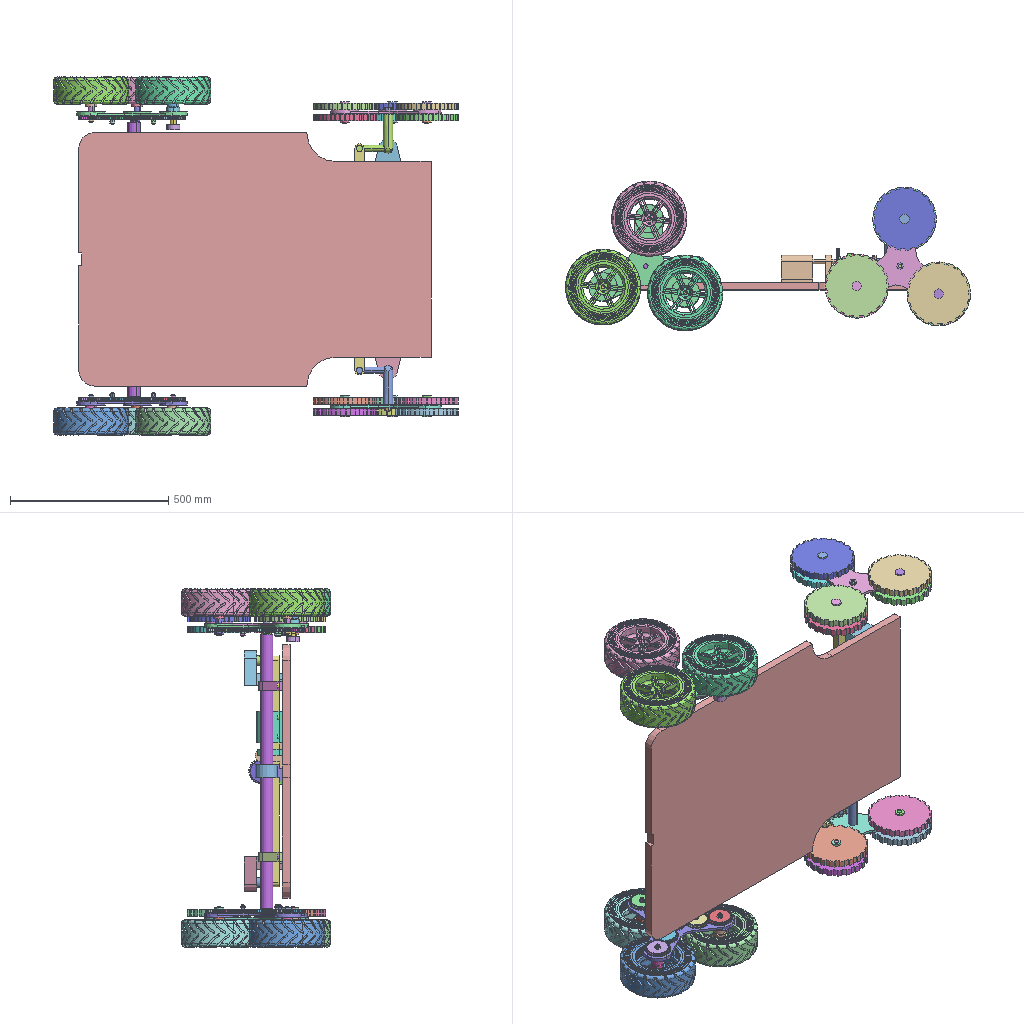Assembly | SolidWorks | 122 different items | 126 placed | box 1278 x 471 x 1130 mm
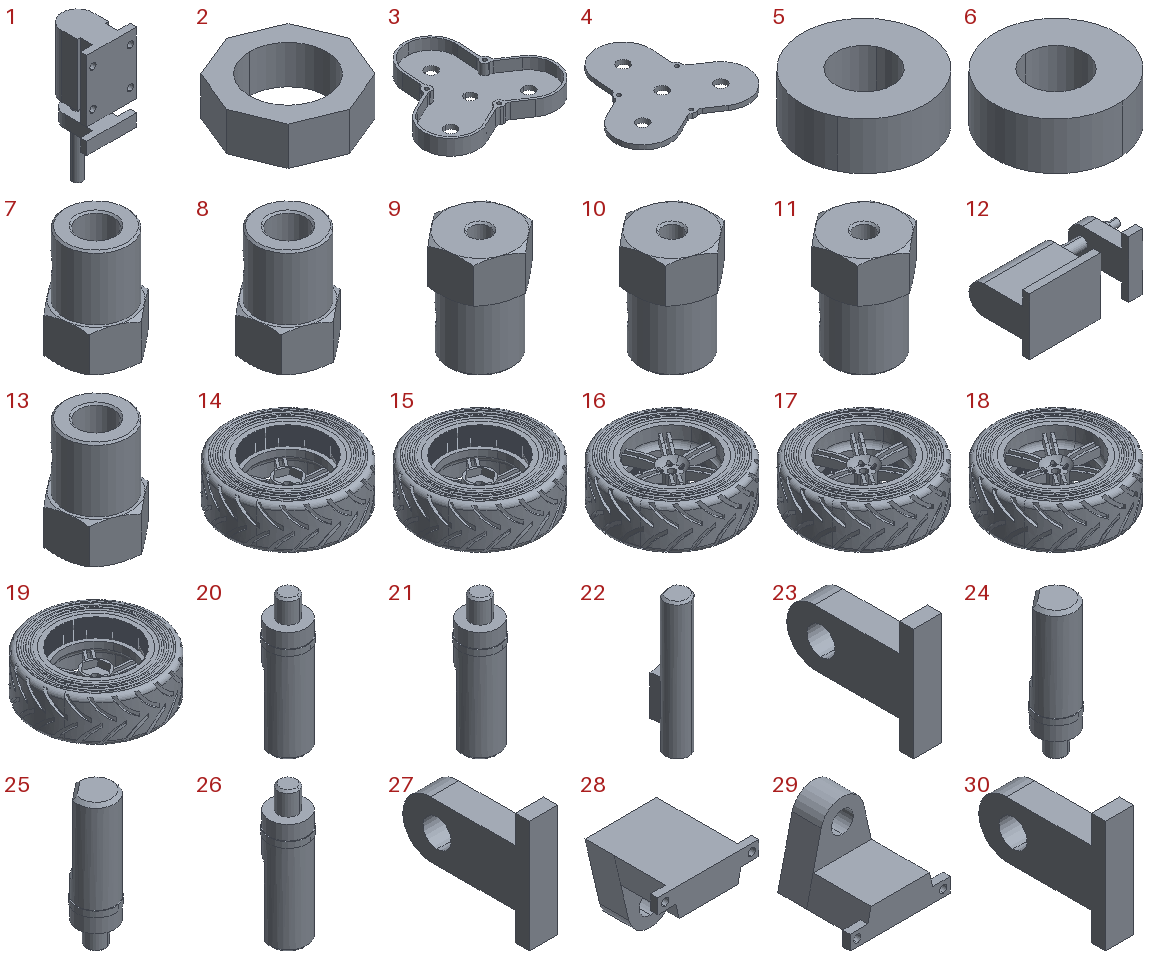Parts list (item | quantity | size | volume | features):
1 | x1 | 80 x 80 x 220 mm | 466808 mm3 | features BaseBody 1
2 | x1 | 16 x 16 x 5 mm | 512.398 mm3 | features BaseBody 1
3 | x1 | 450.446 x 425.125 x 54.4 mm | 2250269 mm3 | features BaseBody 1
4 | x1 | 450.446 x 425.125 x 16 mm | 1740357 mm3 | features BaseBody 1
5 | x1 | 41.6 x 41.6 x 16 mm | 17114 mm3 | features BaseBody 1
6 | x1 | 41.6 x 41.6 x 16 mm | 17114 mm3 | features BaseBody 1
7 | x1 | 41.191 x 43.879 x 57.6 mm | 49620 mm3 | features BaseBody 1
8 | x1 | 41.191 x 43.879 x 57.6 mm | 49620 mm3 | features BaseBody 1
9 | x1 | 41.191 x 43.879 x 57.6 mm | 49620 mm3 | features BaseBody 1
10 | x1 | 41.191 x 43.879 x 57.6 mm | 49620 mm3 | features BaseBody 1
11 | x1 | 41.191 x 43.879 x 57.6 mm | 49620 mm3 | features BaseBody 1
12 | x1 | 188 x 85 x 80 mm | 446040 mm3 | features BaseBody 1
13 | x1 | 41.191 x 43.879 x 57.6 mm | 49620 mm3 | features BaseBody 1
14 | x1 | 236.8 x 236.8 x 86.4 mm | 2369634 mm3 | features BaseBody 1
15 | x1 | 236.8 x 236.8 x 86.4 mm | 2369634 mm3 | features BaseBody 1
16 | x1 | 236.8 x 236.8 x 86.4 mm | 2369635 mm3 | features BaseBody 1
17 | x1 | 236.8 x 236.8 x 86.4 mm | 2369635 mm3 | features BaseBody 1
18 | x1 | 236.8 x 236.8 x 86.4 mm | 2369635 mm3 | features BaseBody 1
19 | x1 | 236.8 x 236.8 x 86.4 mm | 2369634 mm3 | features BaseBody 1
20 | x1 | 20 x 20 x 69.2 mm | 17144 mm3 | features BaseBody 1
21 | x1 | 20 x 20 x 69.2 mm | 17144 mm3 | features BaseBody 1
22 | x1 | 19.2 x 24.894 x 108.8 mm | 33278 mm3 | features BaseBody 1
23 | x1 | 20 x 90 x 80 mm | 70283 mm3 | features BaseBody 1
24 | x1 | 20 x 20 x 69.2 mm | 17144 mm3 | features BaseBody 1
25 | x1 | 20 x 20 x 69.2 mm | 17144 mm3 | features BaseBody 1
26 | x1 | 20 x 20 x 69.2 mm | 17144 mm3 | features BaseBody 1
27 | x1 | 20 x 90 x 80 mm | 70283 mm3 | features BaseBody 1
28 | x1 | 138.517 x 120 x 109.993 mm | 571156 mm3 | features BaseBody 1
29 | x1 | 138.517 x 120 x 109.993 mm | 571156 mm3 | features BaseBody 1
30 | x1 | 20 x 90 x 80 mm | 70283 mm3 | features BaseBody 1
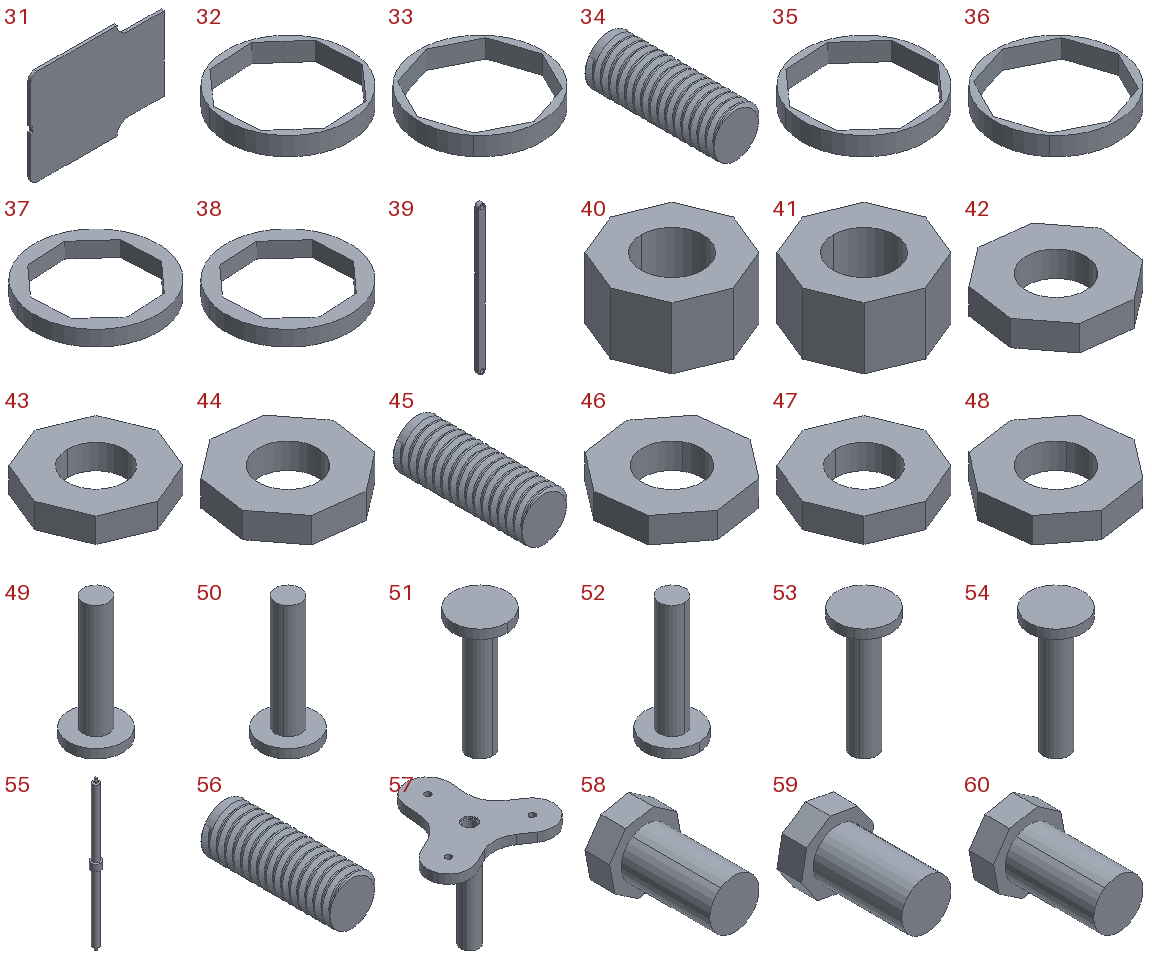31 | x1 | 1112 x 25 x 800 mm | 20489758 mm3 | features BaseBody 1
32 | x1 | 20 x 20 x 3 mm | 176.681 mm3 | features BaseBody 1
33 | x1 | 20 x 20 x 3 mm | 176.681 mm3 | features BaseBody 1
34 | x1 | 6 x 16.008 x 6 mm | 378.104 mm3 | features BaseBody 1
35 | x1 | 20 x 20 x 3 mm | 176.681 mm3 | features BaseBody 1
36 | x1 | 20 x 20 x 3 mm | 176.681 mm3 | features BaseBody 1
37 | x1 | 24 x 24 x 3 mm | 508.64 mm3 | features BaseBody 1
38 | x1 | 24 x 24 x 3 mm | 508.64 mm3 | features BaseBody 1
39 | x1 | 30 x 20 x 730 mm | 420440 mm3 | features BaseBody 1
40 | x1 | 20 x 20 x 10 mm | 2043 mm3 | features BaseBody 1
41 | x1 | 20 x 20 x 10 mm | 2043 mm3 | features BaseBody 1
42 | x1 | 28.978 x 28.978 x 6 mm | 2895 mm3 | features BaseBody 1
43 | x1 | 30 x 30 x 6 mm | 2895 mm3 | features BaseBody 1
44 | x1 | 28.978 x 28.978 x 6 mm | 2895 mm3 | features BaseBody 1
45 | x1 | 6 x 16.008 x 6 mm | 378.104 mm3 | features BaseBody 1
46 | x1 | 28.978 x 28.978 x 6 mm | 2895 mm3 | features BaseBody 1
47 | x1 | 30 x 30 x 6 mm | 2895 mm3 | features BaseBody 1
48 | x1 | 28.978 x 28.978 x 6 mm | 2895 mm3 | features BaseBody 1
49 | x1 | 30 x 30 x 68 mm | 13232 mm3 | features BaseBody 1
50 | x1 | 30 x 30 x 68 mm | 13232 mm3 | features BaseBody 1
51 | x1 | 30 x 30 x 68 mm | 13232 mm3 | features BaseBody 1
52 | x1 | 30 x 30 x 68 mm | 13232 mm3 | features BaseBody 1
53 | x1 | 30 x 30 x 68 mm | 13232 mm3 | features BaseBody 1
54 | x1 | 30 x 30 x 68 mm | 13232 mm3 | features BaseBody 1
55 | x1 | 60 x 60 x 912 mm | 1156729 mm3 | features BaseBody 1
56 | x1 | 6 x 16.008 x 6 mm | 378.104 mm3 | features BaseBody 1
57 | x1 | 199.568 x 186.874 x 175 mm | 351231 mm3 | features BaseBody 1
58 | x1 | 14.681 x 23 x 14.681 mm | 2209 mm3 | features BaseBody 1
59 | x1 | 14.681 x 23 x 14.681 mm | 2209 mm3 | features BaseBody 1
60 | x1 | 14.681 x 23 x 14.681 mm | 2209 mm3 | features BaseBody 1
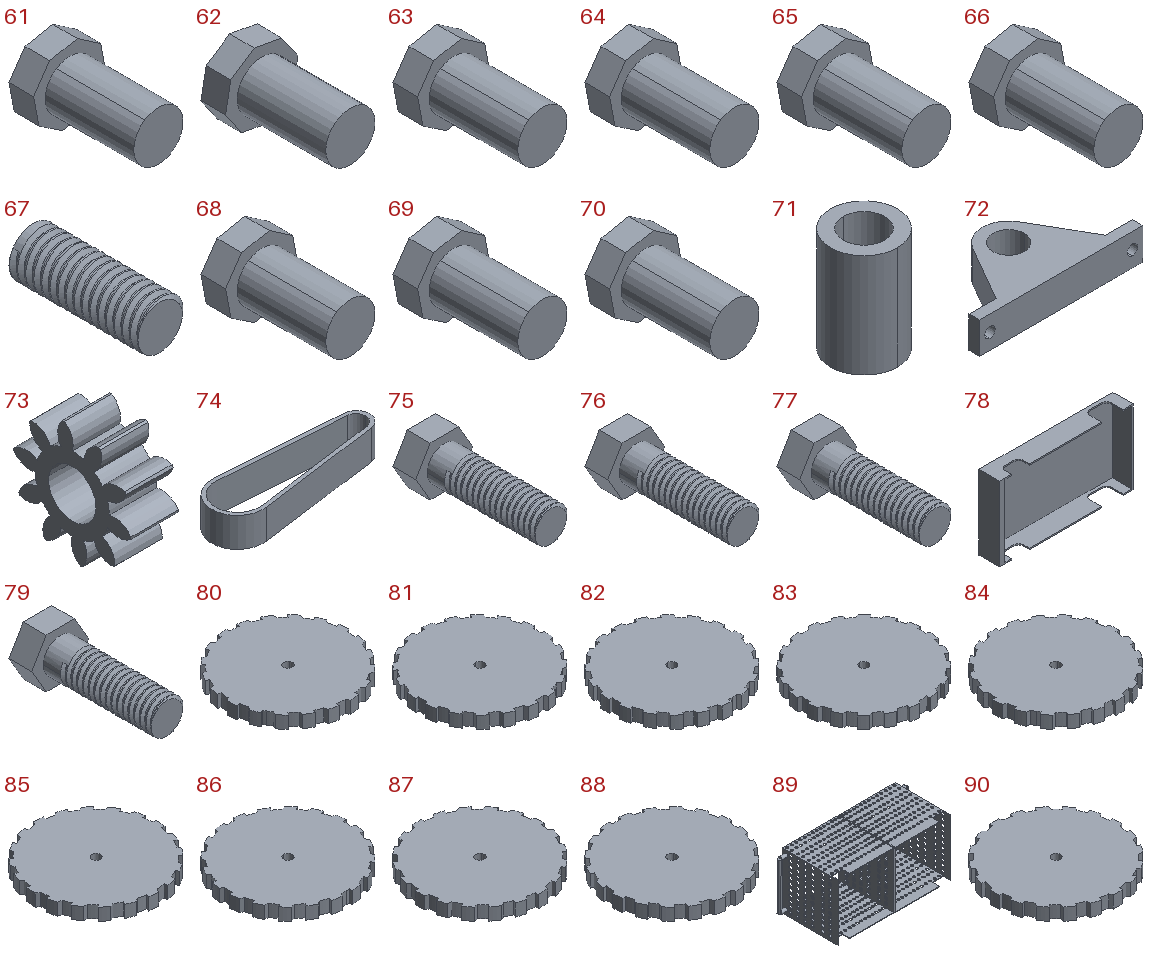61 | x1 | 14.681 x 23 x 14.681 mm | 2209 mm3 | features BaseBody 1
62 | x1 | 14.681 x 23 x 14.681 mm | 2209 mm3 | features BaseBody 1
63 | x1 | 14.681 x 23 x 14.681 mm | 2209 mm3 | features BaseBody 1
64 | x1 | 14.681 x 23 x 14.681 mm | 2209 mm3 | features BaseBody 1
65 | x1 | 14.681 x 23 x 14.681 mm | 2209 mm3 | features BaseBody 1
66 | x1 | 14.681 x 23 x 14.681 mm | 2209 mm3 | features BaseBody 1
67 | x1 | 6 x 16.008 x 6 mm | 378.104 mm3 | features BaseBody 1
68 | x1 | 14.681 x 23 x 14.681 mm | 2209 mm3 | features BaseBody 1
69 | x1 | 14.681 x 23 x 14.681 mm | 2209 mm3 | features BaseBody 1
70 | x1 | 14.681 x 23 x 14.681 mm | 2209 mm3 | features BaseBody 1
71 | x1 | 26 x 26 x 40 mm | 13195 mm3 | features BaseBody 1
72 | x1 | 155.5 x 75 x 30 mm | 151396 mm3 | features BaseBody 1
73 | x1 | - | - | features RefSurface 1
74 | x1 | 219.551 x 70 x 40 mm | 97158 mm3 | features BaseBody 1
75 | x1 | 10 x 23 x 8.66 mm | 722.509 mm3 | features BaseBody 1
76 | x1 | 10 x 23 x 8.66 mm | 722.509 mm3 | features BaseBody 1
77 | x1 | 10 x 23 x 8.66 mm | 722.509 mm3 | features BaseBody 1
78 | x1 | 1112 x 170.835 x 618 mm | 11764605 mm3 | features BaseBody 1
79 | x1 | 10 x 23 x 8.66 mm | 722.509 mm3 | features BaseBody 1
80 | x1 | 199.988 x 199.988 x 20 mm | 595746 mm3 | features BaseBody 1
81 | x1 | 199.75 x 199.75 x 20 mm | 595746 mm3 | features BaseBody 1
82 | x1 | 199.947 x 199.947 x 20 mm | 595746 mm3 | features BaseBody 1
83 | x1 | 199.408 x 199.408 x 20 mm | 595746 mm3 | features BaseBody 1
84 | x1 | 200 x 200 x 20 mm | 595746 mm3 | features BaseBody 1
85 | x1 | 200 x 200 x 20 mm | 595746 mm3 | features BaseBody 1
86 | x1 | 199.75 x 199.75 x 20 mm | 595746 mm3 | features BaseBody 1
87 | x1 | 200 x 200 x 20 mm | 595746 mm3 | features BaseBody 1
88 | x1 | 199.857 x 199.857 x 20 mm | 595746 mm3 | features BaseBody 1
89 | x1 | 1140 x 495 x 500 mm | 8546977 mm3 | features BaseBody 1
90 | x1 | 200 x 200 x 20 mm | 595746 mm3 | features BaseBody 1
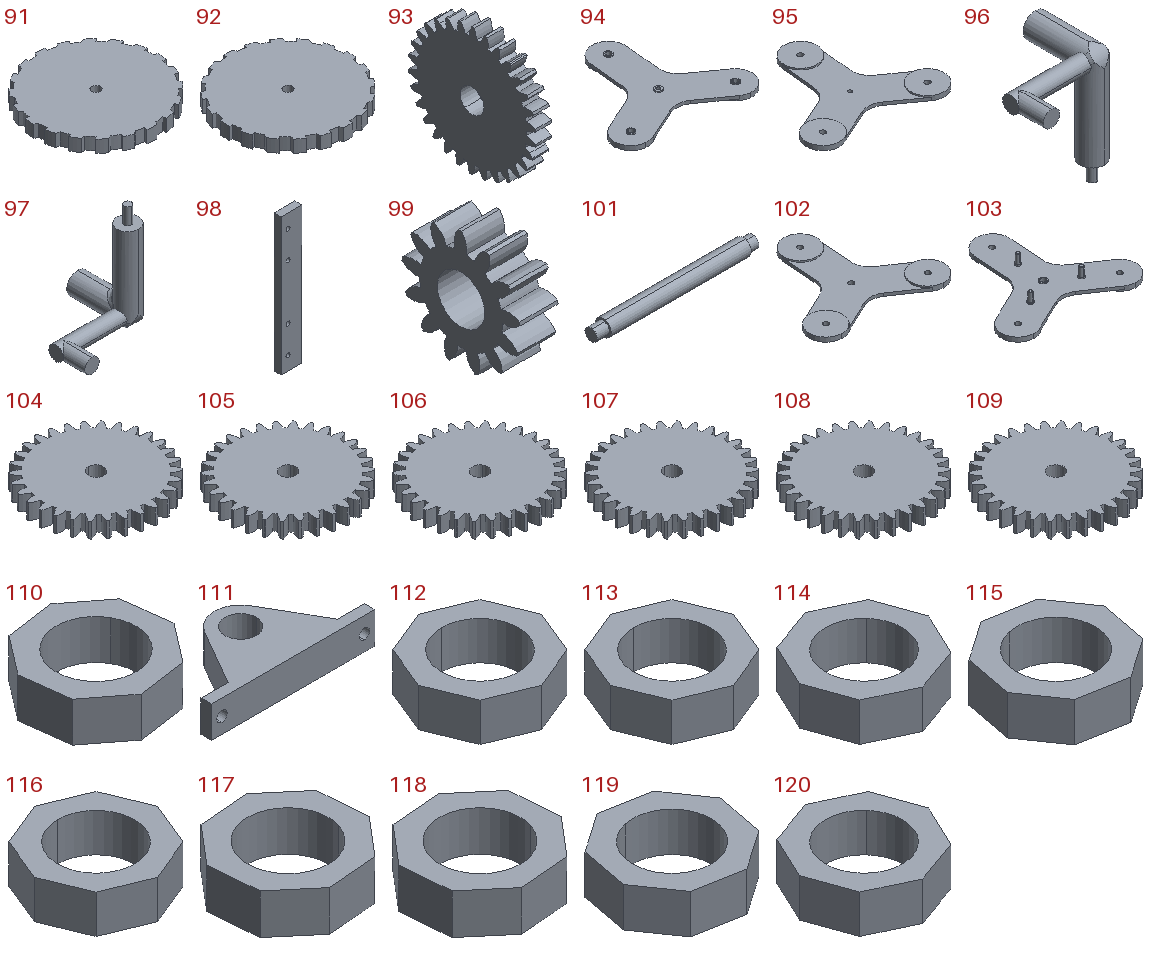91 | x1 | 199.988 x 199.988 x 20 mm | 595746 mm3 | features BaseBody 1
92 | x1 | 200 x 200 x 20 mm | 595746 mm3 | features BaseBody 1
93 | x1 | - | - | features RefSurface 1
94 | x1 | 348.636 x 326.309 x 15 mm | 447458 mm3 | features BaseBody 1
95 | x1 | 348.636 x 326.309 x 15 mm | 447458 mm3 | features BaseBody 1
96 | x1 | 115 x 110 x 145 mm | 163040 mm3 | features BaseBody 1
97 | x1 | 115 x 110 x 145 mm | 163040 mm3 | features BaseBody 1
98 | x1 | 30 x 10 x 200 mm | 58869 mm3 | features BaseBody 1
99 | x1 | - | - | features RefSurface 1
100 | x1 | - | - | features BaseBody 1
101 | x1 | 200 x 20 x 20 mm | 59121 mm3 | features BaseBody 1
102 | x1 | 349.137 x 323.748 x 39 mm | 452459 mm3 | features BaseBody 1
103 | x1 | 349.137 x 323.748 x 39 mm | 452459 mm3 | features BaseBody 1
104 | x4 | - | - | features RefSurface 1
105 | x1 | - | - | features RefSurface 1
106 | x1 | - | - | features RefSurface 1
107 | x1 | - | - | features RefSurface 1
108 | x1 | - | - | features RefSurface 1
109 | x2 | - | - | features RefSurface 1
110 | x1 | 15.455 x 15.455 x 5 mm | 512.398 mm3 | features BaseBody 1
111 | x1 | 155.5 x 75 x 30 mm | 151396 mm3 | features BaseBody 1
112 | x1 | 16 x 16 x 5 mm | 512.398 mm3 | features BaseBody 1
113 | x1 | 16 x 16 x 5 mm | 512.398 mm3 | features BaseBody 1
114 | x1 | 15.981 x 15.981 x 5 mm | 512.398 mm3 | features BaseBody 1
115 | x1 | 15.639 x 15.639 x 5 mm | 512.398 mm3 | features BaseBody 1
116 | x1 | 16 x 16 x 5 mm | 512.398 mm3 | features BaseBody 1
117 | x1 | 15.234 x 15.234 x 5 mm | 512.398 mm3 | features BaseBody 1
118 | x1 | 15.234 x 15.234 x 5 mm | 512.398 mm3 | features BaseBody 1
119 | x1 | 15.639 x 15.639 x 5 mm | 512.398 mm3 | features BaseBody 1
120 | x1 | 15.981 x 15.981 x 5 mm | 512.398 mm3 | features BaseBody 1
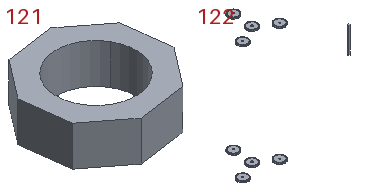121 | x1 | 15.455 x 15.455 x 5 mm | 512.398 mm3 | features BaseBody 1
122 | x1 | - | - | features RefSurface 9
Mates (type | each side: item.copy, entity, surface, feature):
Concentric | 103.1 face cylinder 输入1 | 109.1 face cylinder 曲Face-输入1
Coincident | 109.2 face plane 曲Face-输入1 | 109.1 face plane 曲Face-输入1
Concentric | 103.1 face cylinder 输入1 | 104.1 face cylinder 曲Face-输入1
Coincident | 104.2 face plane 曲Face-输入1 | 104.1 face plane 曲Face-输入1
Concentric | 103.1 face cylinder 输入1 | 104.3 face cylinder 曲Face-输入1
Coincident | 104.2 face plane 曲Face-输入1 | 104.3 face plane 曲Face-输入1
Concentric | 103.1 face cylinder 输入1 | 104.4 face cylinder 曲Face-输入1
Coincident | 105.1 face plane 曲Face-输入1 | 104.4 face plane 曲Face-输入1